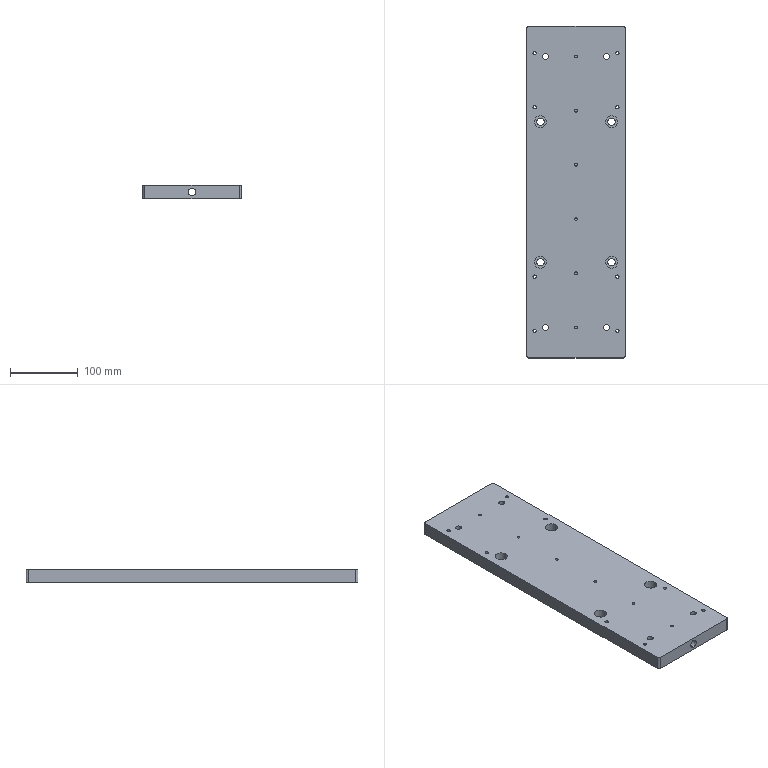Part | STEP file | LM-05-1224B_default | 1 solid | 88 faces | box 145 x 490 x 20 mm | volume 1346383 mm3 | cylinder 70 | plane 14 | cone 4 | commonest cylinder face diameters 5 x16 4 x12 8.5 x8 11 x8 18 x8 30 x8